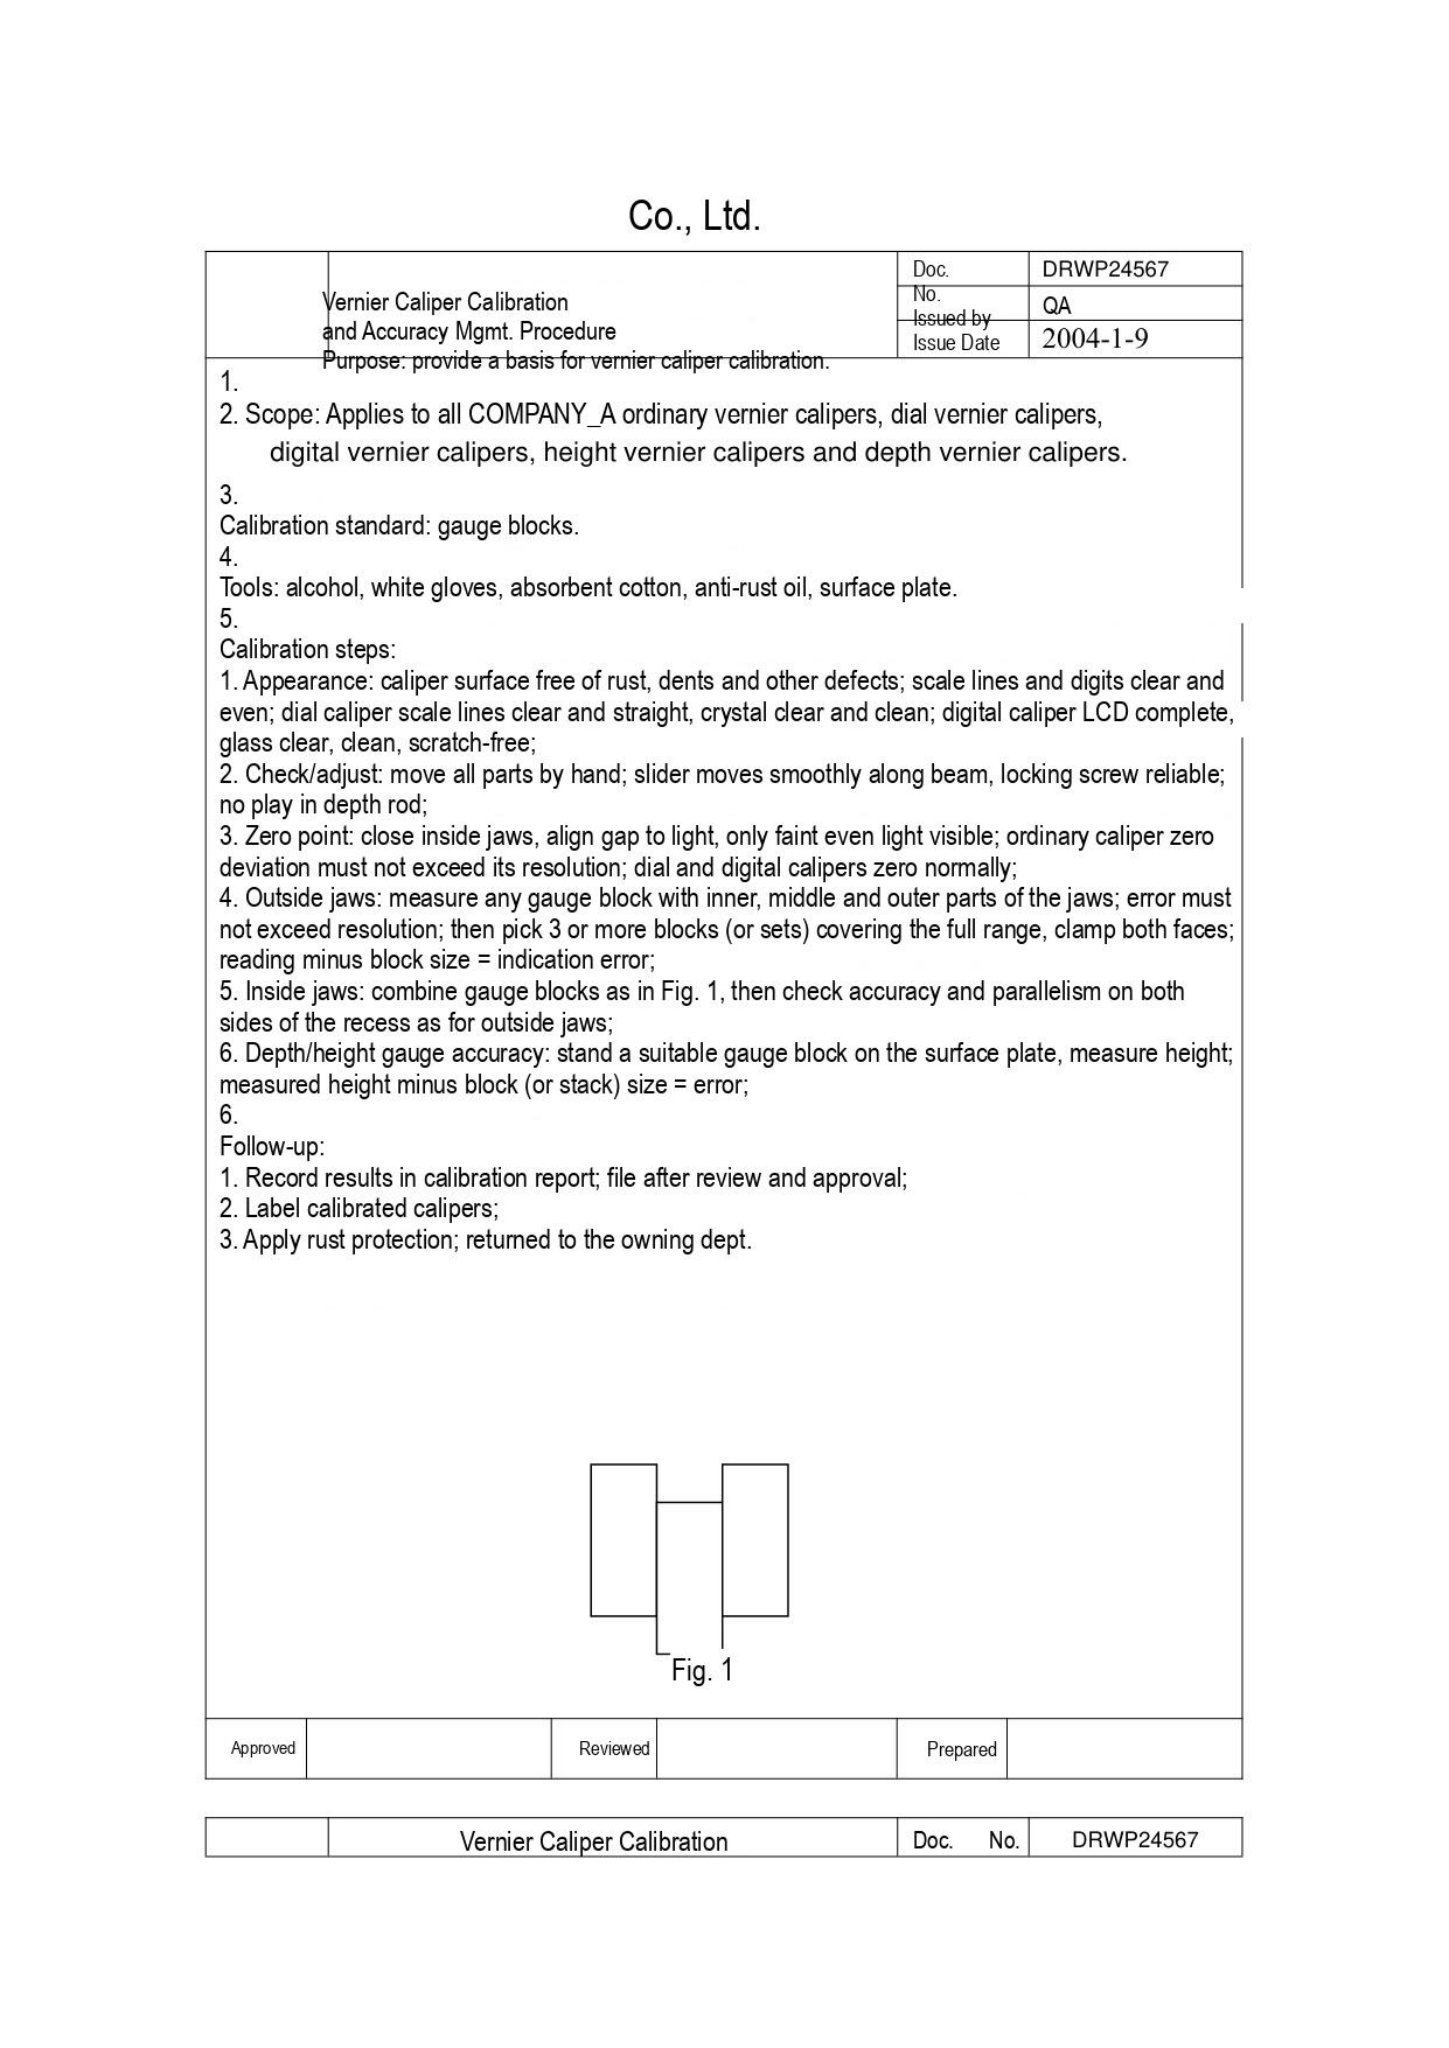Co., Ltd.

| | Vernier Caliper Calibration and Accuracy Mgmt. Procedure | Doc. No. | DRWP24567 |
|---|---|---|---|
| | | Issued by | QA |
| | | Issue Date | 2004-1-9 |

Purpose: provide a basis for vernier caliper calibration.

1.

2. Scope: Applies to all COMPANY_A ordinary vernier calipers, dial vernier calipers, digital vernier calipers, height vernier calipers and depth vernier calipers.

3.

Calibration standard: gauge blocks.

4.

Tools: alcohol, white gloves, absorbent cotton, anti-rust oil, surface plate.

5.

Calibration steps:

1. Appearance: caliper surface free of rust, dents and other defects; scale lines and digits clear and even; dial caliper scale lines clear and straight, crystal clear and clean; digital caliper LCD complete, glass clear, clean, scratch-free;

2. Check/adjust: move all parts by hand; slider moves smoothly along beam, locking screw reliable; no play in depth rod;

3. Zero point: close inside jaws, align gap to light, only faint even light visible; ordinary caliper zero deviation must not exceed its resolution; dial and digital calipers zero normally;

4. Outside jaws: measure any gauge block with inner, middle and outer parts of the jaws; error must not exceed resolution; then pick 3 or more blocks (or sets) covering the full range, clamp both faces; reading minus block size = indication error;

5. Inside jaws: combine gauge blocks as in Fig. 1, then check accuracy and parallelism on both sides of the recess as for outside jaws;

6. Depth/height gauge accuracy: stand a suitable gauge block on the surface plate, measure height; measured height minus block (or stack) size = error;

6.

Follow-up:

1. Record results in calibration report; file after review and approval;

2. Label calibrated calipers;

3. Apply rust protection; returned to the owning dept.

Fig. 1

| Approved | | Reviewed | | Prepared | |
|---|---|---|---|---|---|

| | Vernier Caliper Calibration | Doc. No. | DRWP24567 |
|---|---|---|---|
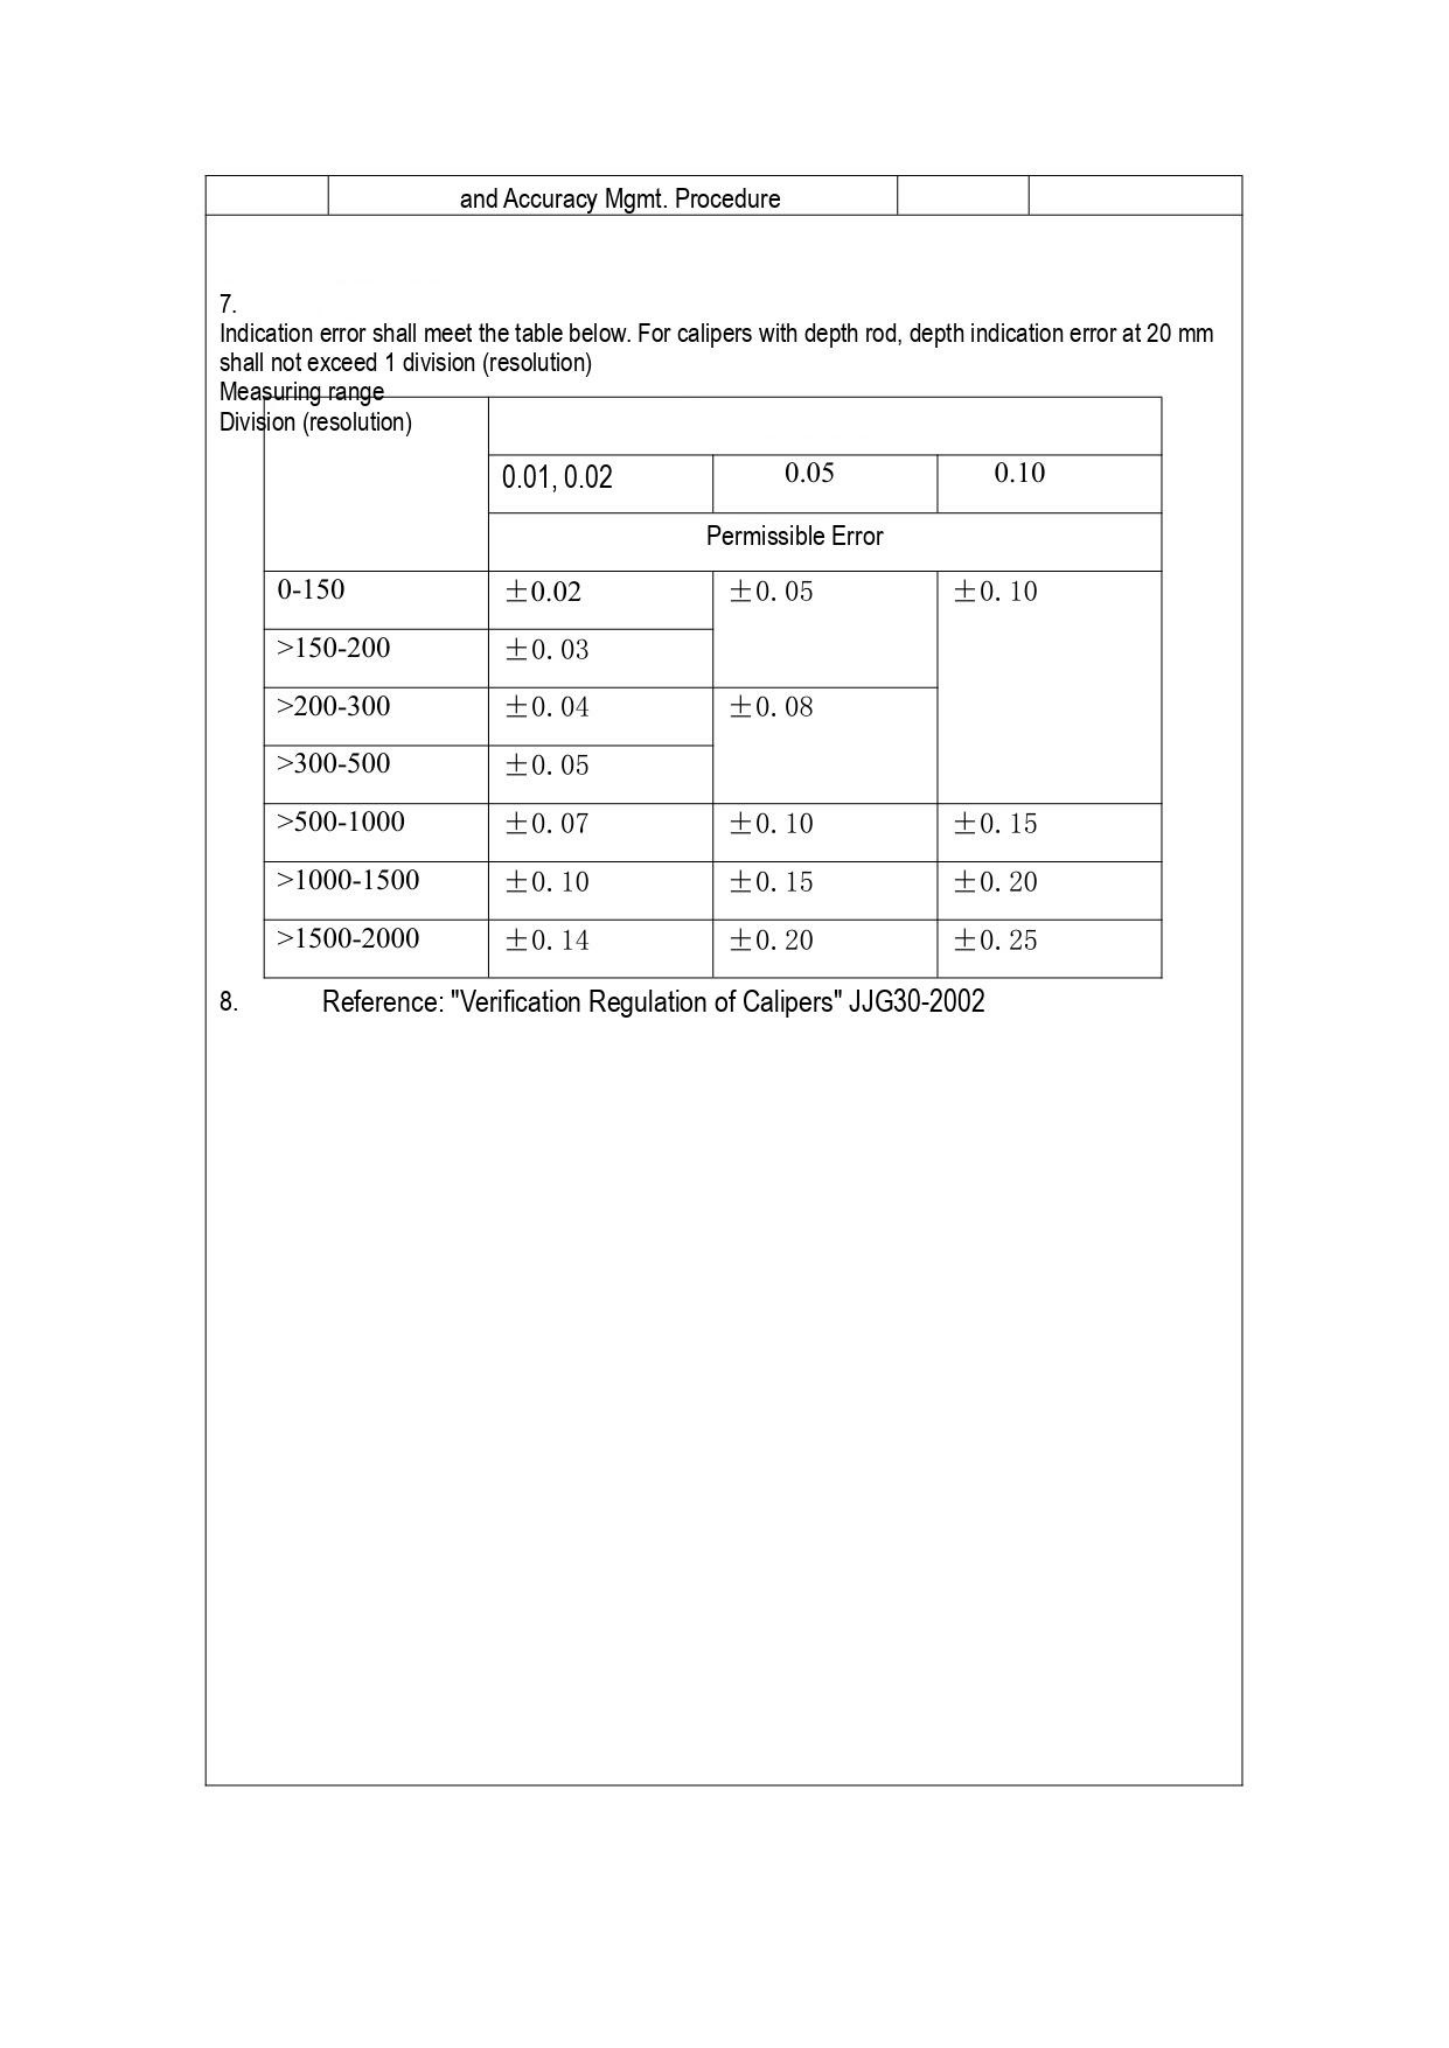| | and Accuracy Mgmt. Procedure | | |
|---|---|---|---|

7.
Indication error shall meet the table below. For calipers with depth rod, depth indication error at 20 mm shall not exceed 1 division (resolution)
Measuring range
Division (resolution)

| | | | |
|---|---|---|---|
| | 0.01, 0.02 | 0.05 | 0.10 |
| | Permissible Error | | |
| 0-150 | ±0.02 | ±0. 05 | ±0. 10 |
| >150-200 | ±0. 03 | | |
| >200-300 | ±0. 04 | ±0. 08 | |
| >300-500 | ±0. 05 | | |
| >500-1000 | ±0. 07 | ±0. 10 | ±0. 15 |
| >1000-1500 | ±0. 10 | ±0. 15 | ±0. 20 |
| >1500-2000 | ±0. 14 | ±0. 20 | ±0. 25 |

8. Reference: "Verification Regulation of Calipers" JJG30-2002